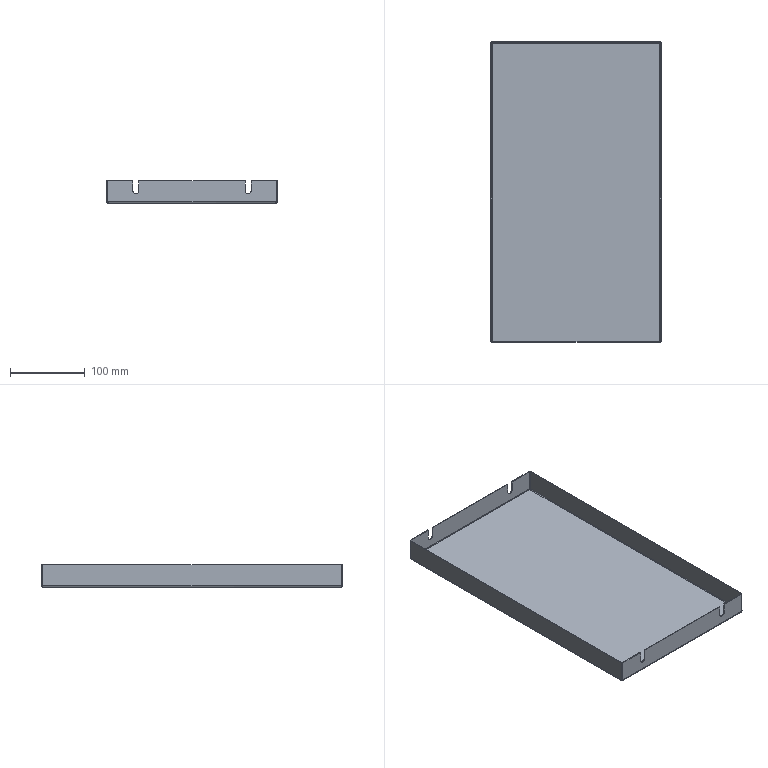Part | 1 solid | 54 faces | box 228 x 402 x 30 mm | volume 151642 mm3 | plane 34 | cylinder 12 | spline 8 | commonest cylinder face diameters 1.473 x4 3.873 x4 8.2 x4